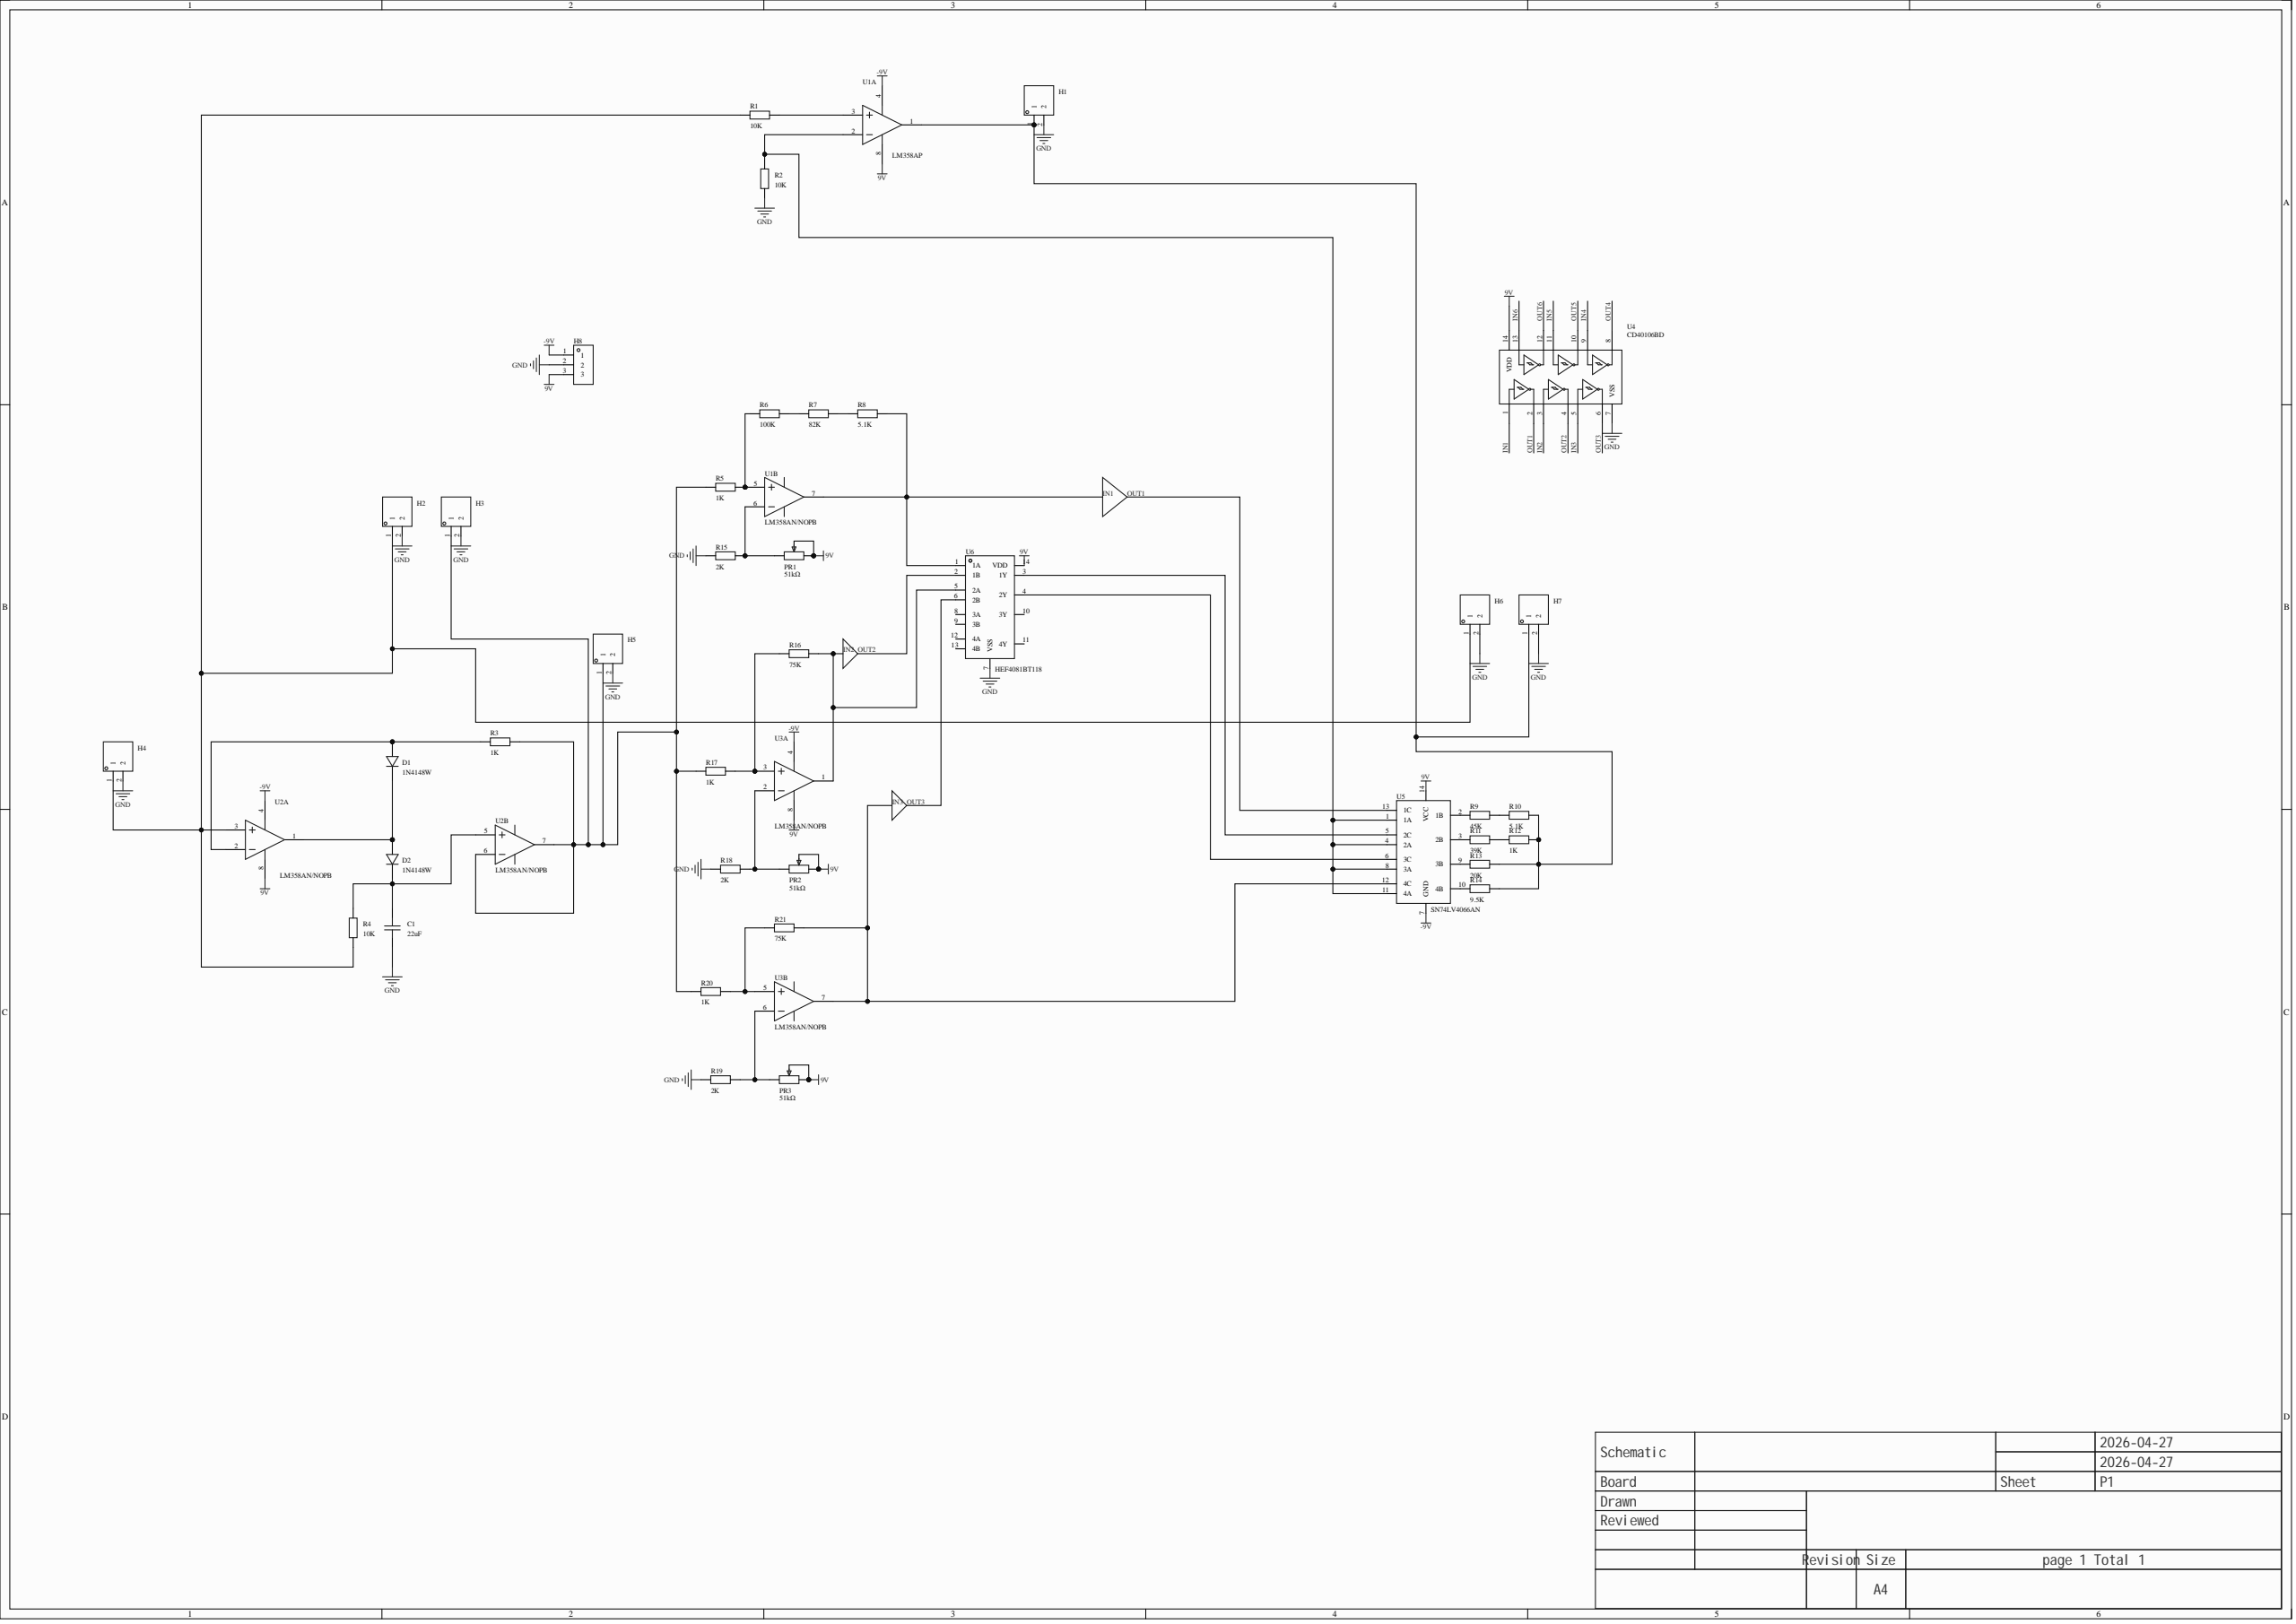Circuit board | Altium Designer | 41 parts | 33 nets
Bill of materials:
Comment,Description,Designator,Footprint,LibRef,Quantity
"22uF","","C1","CAP-TH_L5.0-W2.5-P5.00-D1.0","CAP_0603","1"
"1N4148W","Diode configuration: independent; forward voltage (Vf): 1V@50mA; DC reverse voltage (Vr): 75V; rectified current: 150mA; reverse recovery time (Trr): 4ns;","D1, D2","SOD-123F_L2.7-W1.6-LS3.8-RD","1N4148W_C81598","2"
"","","H1, H2, H3, H4, H5, H6, H7","HDR-TH_2P-P2.54-V-M-1","HDR-M_2.54_1x2P","7"
"","","H8","HDR-TH_3P-P2.54-V-F","HDR-F_2.54_1x3P","1"
"51kΩ","","PR1, PR2, PR3","R_3296","R_3296","3"
"10K","","R1, R2, R4","Res_1/8W","Res_0603","3"
"1K","","R3, R5, R12, R17, R20","Res_1/8W","Res_0603","5"
"100K","","R6","Res_1/8W","Res_0603","1"
"82K","","R7","Res_1/8W","Res_0603","1"
"5.1K","","R8, R10","Res_1/8W","Res_0603","2"
"45K","","R9","Res_1/8W","Res_0603","1"
"39K","","R11","Res_1/8W","Res_0603","1"
"20K","","R13","Res_1/8W","Res_0603","1"
"9.5K","","R14","Res_1/8W","Res_0603","1"
"2K","","R15, R18, R19","Res_1/8W","Res_0603","3"
"75K","","R16, R21","Res_1/8W","Res_0603","2"
"LM358AP","Amplifiers: 2; rail-to-rail: -; GBW: 1MHz; input offset voltage (Vos): 2mV; slew rate (SR): -; input bias current (Ib): 50nA;","U1","PDIP-8_L10.2-W6.5-P2.54-LS7.6-BL","LM358AN/NOPB","1"
"LM358AN/NOPB","Amplifiers: 2; rail-to-rail: -; GBW: 1MHz; input offset voltage (Vos): 2mV; slew rate (SR): -; input bias current (Ib): 50nA;","U2, U3","PDIP-8_L10.2-W6.5-P2.54-LS7.6-BL","LM358AN/NOPB","2"
"CD40106BD","Input type: Schmitt trigger; operating voltage: 3V~15V; quiescent current (Iq): 16uA; channels: 6; propagation delay (tpd): 80ns@10V, 50pF; 70ns@15V, 50pF; 220ns@5V, 50pF;","U4","DIP-14_L19.1-W6.4-P2.54-LS7.6-BL","CD40106BD","1"
"SN74LV4066AN","Switch circuit: SPST-NO; channels: 4; on-resistance (Ron@VCC): 75Ω;","U5","PDIP-14_L19.3-W6.4-P2.54-LS7.9-BL-1","SN74LV4066AN","1"
"HEF4081BT118","Logic type: AND gate; channels: 4; operating voltage: 3V~15V; quiescent current (Iq): 1uA; propagation delay (tpd): 50ns@10V, 50pF; 110ns@5V, 50pF; 40ns@15V, 50pF;","U6","SO-14_L8.9-W3.9-P1.27-LS6.0-BL","HEF4081BT118","1"
Netlist (Protel format):
[
C1
CAP-TH_L5.0-W2.5-P5.00-D1.0
22uF



]
[
D1
SOD-123F_L2.7-W1.6-LS3.8-RD
1N4148W



]
[
D2
SOD-123F_L2.7-W1.6-LS3.8-RD
1N4148W



]
[
H1
HDR-TH_2P-P2.54-V-M-1




]
[
H2
HDR-TH_2P-P2.54-V-M-1




]
[
H3
HDR-TH_2P-P2.54-V-M-1




]
[
H4
HDR-TH_2P-P2.54-V-M-1




]
[
H5
HDR-TH_2P-P2.54-V-M-1




]
[
H6
HDR-TH_2P-P2.54-V-M-1




]
[
H7
HDR-TH_2P-P2.54-V-M-1




]
[
H8
HDR-TH_3P-P2.54-V-F




]
[
PR1
R_3296
51kΩ



]
[
PR2
R_3296
51kΩ



]
[
PR3
R_3296
51kΩ



]
[
R1
Res_1/8W
10K



]
[
R2
Res_1/8W
10K



]
[
R3
Res_1/8W
1K



]
[
R4
Res_1/8W
10K



]
[
R5
Res_1/8W
1K



]
[
R6
Res_1/8W
100K



]
[
R7
Res_1/8W
82K



]
[
R8
Res_1/8W
5.1K



]
[
R9
Res_1/8W
45K



]
[
R10
Res_1/8W
5.1K



]
[
R11
Res_1/8W
39K



]
[
R12
Res_1/8W
1K



]
[
R13
Res_1/8W
20K



]
[
R14
Res_1/8W
9.5K



]
[
R15
Res_1/8W
2K



]
[
R16
Res_1/8W
75K



]
[
R17
Res_1/8W
1K



]
[
R18
Res_1/8W
2K



]
[
R19
Res_1/8W
2K



]
[
R20
Res_1/8W
1K



]
[
R21
Res_1/8W
75K



]
[
U1
PDIP-8_L10.2-W6.5-P2.54-LS7.6-BL
LM358AP



]
[
U2
PDIP-8_L10.2-W6.5-P2.54-LS7.6-BL
LM358AN/NOPB



]
[
U3
PDIP-8_L10.2-W6.5-P2.54-LS7.6-BL
LM358AN/NOPB



]
[
U4
DIP-14_L19.1-W6.4-P2.54-LS7.6-BL
CD40106BD



]
[
U5
PDIP-14_L19.3-W6.4-P2.54-LS7.9-BL-1
SN74LV4066AN



]
[
U6
SO-14_L8.9-W3.9-P1.27-LS6.0-BL
HEF4081BT118



]
(
OUT3
U4-6
U6-6
)
(
OUT2
U4-4
U6-2
)
(
OUT1
U4-2
U5-13
)
(
NetU5_6
U5-6
U6-4
)
(
NetU5_5
U5-5
U6-3
)
(
NetR20_2
R20-2
R21-1
U3-5
)
(
NetR16_1
R16-1
R17-2
U3-3
)
(
NetR14_1
R14-1
U5-10
)
(
NetR13_1
R13-1
U5-9
)
(
NetR11_2
R11-2
R12-1
)
(
NetR11_1
R11-1
U5-3
)
(
NetR9_2
R9-2
R10-1
)
(
NetR9_1
R9-1
U5-2
)
(
NetR7_2
R7-2
R8-1
)
(
NetR6_2
R6-2
R7-1
)
(
NetR5_2
R5-2
R6-1
U1-5
)
(
NetR2_2
R2-2
U1-2
U5-1
U5-4
U5-8
U5-11
)
(
NetR1_2
R1-2
U1-3
)
(
NetPR3_3
PR3-3
R19-2
U3-6
)
(
NetPR2_3
PR2-3
R18-2
U3-2
)
(
NetPR1_3
PR1-3
R15-2
U1-6
)
(
NetH3_1
H3-1
H5-1
R3-2
R5-1
R17-1
R20-1
U2-6
U2-7
)
(
NetH2_1
H2-1
H4-1
H6-1
R1-1
R4-1
U2-3
)
(
NetH1_1
H1-1
H7-1
R10-2
R12-2
R13-2
R14-2
U1-1
)
(
NetD1_2
D1-2
R3-1
U2-2
)
(
NetD1_1
D1-1
D2-2
U2-1
)
(
NetC1_2
C1-2
D2-1
R4-2
U2-5
)
(
IN3
R21-2
U3-7
U4-5
U5-12
)
(
IN2
R16-2
U3-1
U4-3
U6-5
)
(
IN1
R8-2
U1-7
U4-1
U6-1
)
(
GND
C1-1
H1-2
H2-2
H3-2
H4-2
H5-2
H6-2
H7-2
H8-2
R2-1
R15-1
R18-1
R19-1
U4-7
U6-7
)
(
-9V
H8-1
U1-4
U2-4
U3-4
U5-7
)
(
9V
H8-3
PR1-1
PR1-2
PR2-1
PR2-2
PR3-1
PR3-2
U1-8
U2-8
U3-8
U4-14
U5-14
U6-14
)